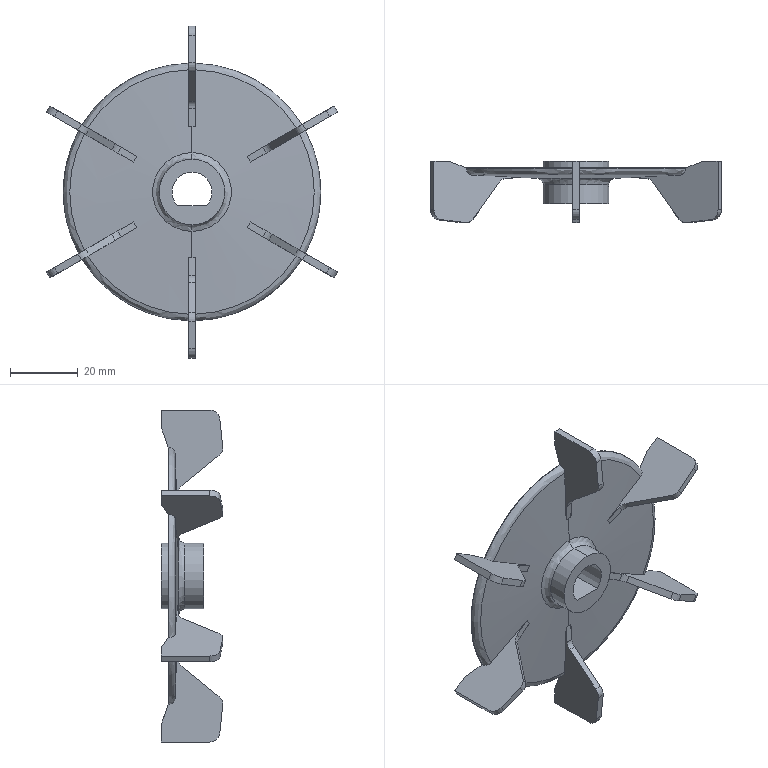Part | SolidWorks | features BaseBody 1 | 1 solid | 120 faces | box 85.87 x 18.15 x 98 mm | volume 14348 mm3 | plane 75 | cylinder 23 | spline 16 | cone 6 | commonest cylinder face diameters 6 x18 19.4 x4 11.8 x1